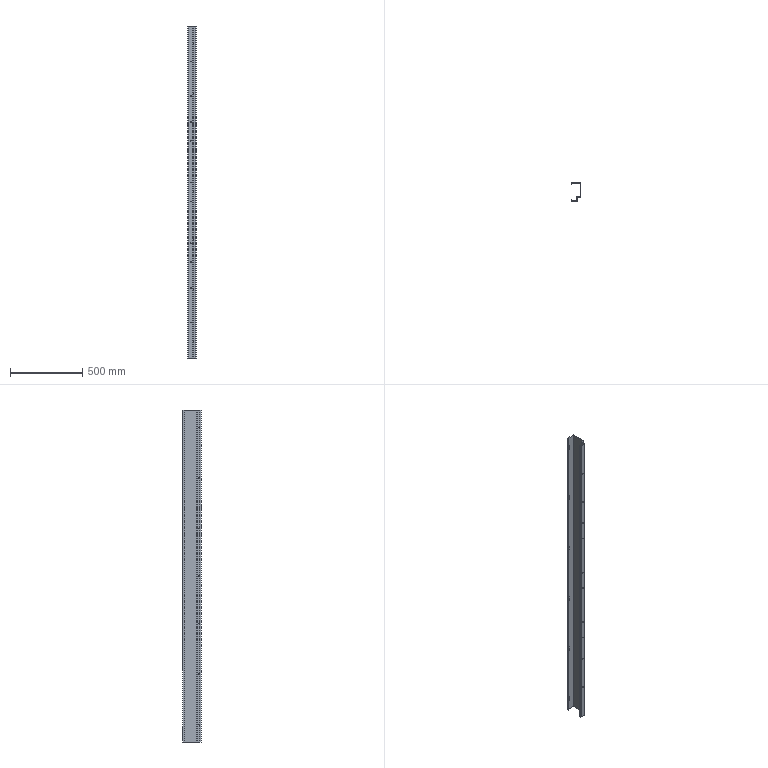Part | 1 solid | 118 faces | box 58 x 130 x 2300 mm | volume 718321 mm3 | cylinder 64 | plane 54 | commonest cylinder face diameters 5 x20 9 x18 4.6 x14 2 x6 4.4 x6